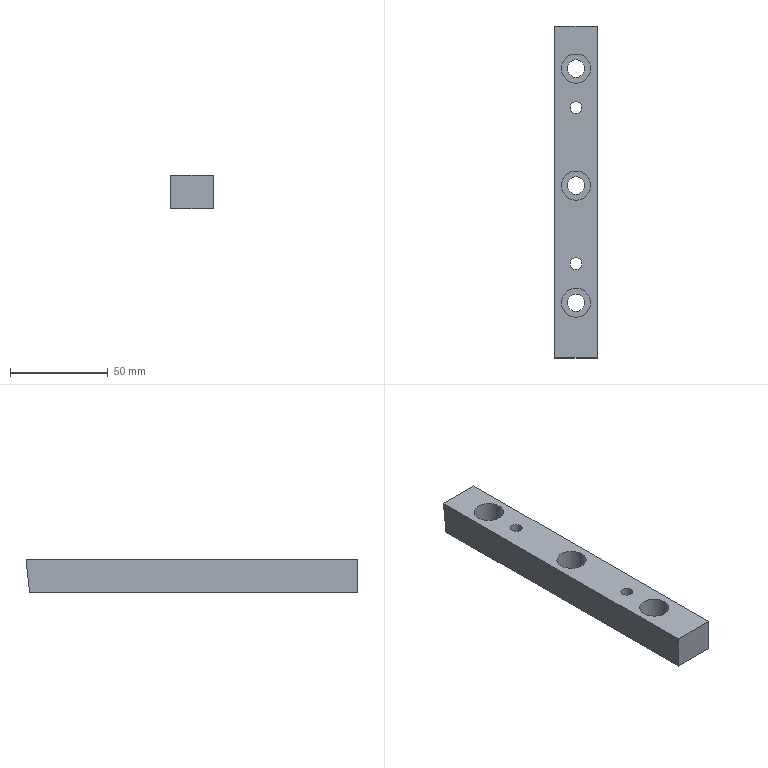Part | NX | features DATUM_CSYS 4, CBORE_HOLE 3, SKETCH 3, HOLE PACKAGE 2, SIMPLE HOLE 2, EXTRUDE 1 | 1 solid | 17 faces | box 22 x 170.1 x 17 mm | volume 55003 mm3 | plane 9 | cylinder 8 | commonest cylinder face diameters 9 x3 15 x3 6 x2
STEP:
#1=CARTESIAN_POINT('',(0.,-85.05,8.5));
#2=VERTEX_POINT('',#1);
#3=CARTESIAN_POINT('',(0.,-85.05,-8.5));
#4=VERTEX_POINT('',#3);
#5=CARTESIAN_POINT('',(0.,-85.05,8.5));
#6=DIRECTION('',(0.,0.,-1.));
#7=VECTOR('',#6,1000.);
#8=LINE('',#5,#7);
#9=EDGE_CURVE('',#2,#4,#8,.T.);
#10=ORIENTED_EDGE('',*,*,#9,.T.);
#11=CARTESIAN_POINT('',(22.,-85.05,-8.5));
#12=VERTEX_POINT('',#11);
#13=CARTESIAN_POINT('',(22.,-85.05,-8.5));
#14=DIRECTION('',(-1.,0.,0.));
#15=VECTOR('',#14,1000.);
#16=LINE('',#13,#15);
#17=EDGE_CURVE('',#12,#4,#16,.T.);
#18=ORIENTED_EDGE('',*,*,#17,.F.);
#19=CARTESIAN_POINT('',(22.,-85.05,8.5));
#20=VERTEX_POINT('',#19);
#21=CARTESIAN_POINT('',(22.,-85.05,8.5));
#22=DIRECTION('',(0.,0.,-1.));
#23=VECTOR('',#22,1000.);
#24=LINE('',#21,#23);
#25=EDGE_CURVE('',#20,#12,#24,.T.);
#26=ORIENTED_EDGE('',*,*,#25,.F.);
#27=CARTESIAN_POINT('',(22.,-85.05,8.5));
#28=DIRECTION('',(-1.,0.,0.));
#29=VECTOR('',#28,1000.);
#30=LINE('',#27,#29);
#31=EDGE_CURVE('',#20,#2,#30,.T.);
#32=ORIENTED_EDGE('',*,*,#31,.T.);
#33=EDGE_LOOP('',(#10,#18,#26,#32));
#34=FACE_BOUND('',#33,.T.);
#35=CARTESIAN_POINT('',(22.,-85.05,8.5));
#36=DIRECTION('',(0.,1.,0.));
#37=DIRECTION('',(0.,0.,1.));
#38=AXIS2_PLACEMENT_3D('',#35,#36,#37);
#39=PLANE('',#38);
#40=ADVANCED_FACE('',(#34),#39,.F.);
#41=CARTESIAN_POINT('',(14.,43.25,-8.5));
#42=VERTEX_POINT('',#41);
#43=CARTESIAN_POINT('',(11.,43.25,-8.5));
#44=DIRECTION('',(0.,0.,1.));
#45=DIRECTION('',(1.,0.,0.));
#46=AXIS2_PLACEMENT_3D('',#43,#44,#45);
#47=CIRCLE('',#46,3.);
#48=EDGE_CURVE('',#42,#42,#47,.T.);
#49=ORIENTED_EDGE('',*,*,#48,.T.);
#50=EDGE_LOOP('',(#49));
#51=FACE_BOUND('',#50,.T.);
#52=CARTESIAN_POINT('',(14.,-36.75,-8.5));
#53=VERTEX_POINT('',#52);
#54=CARTESIAN_POINT('',(11.,-36.75,-8.5));
#55=DIRECTION('',(0.,0.,1.));
#56=DIRECTION('',(1.,0.,0.));
#57=AXIS2_PLACEMENT_3D('',#54,#55,#56);
#58=CIRCLE('',#57,3.);
#59=EDGE_CURVE('',#53,#53,#58,.T.);
#60=ORIENTED_EDGE('',*,*,#59,.T.);
#61=EDGE_LOOP('',(#60));
#62=FACE_BOUND('',#61,.T.);
#63=CARTESIAN_POINT('',(15.5,63.25,-8.5));
#64=VERTEX_POINT('',#63);
#65=CARTESIAN_POINT('',(11.,63.25,-8.5));
#66=DIRECTION('',(0.,0.,1.));
#67=DIRECTION('',(1.,0.,0.));
#68=AXIS2_PLACEMENT_3D('',#65,#66,#67);
#69=CIRCLE('',#68,4.5);
#70=EDGE_CURVE('',#64,#64,#69,.T.);
#71=ORIENTED_EDGE('',*,*,#70,.T.);
#72=EDGE_LOOP('',(#71));
#73=FACE_BOUND('',#72,.T.);
#74=CARTESIAN_POINT('',(15.5,3.25,-8.5));
#75=VERTEX_POINT('',#74);
#76=CARTESIAN_POINT('',(11.,3.25,-8.5));
#77=DIRECTION('',(0.,0.,1.));
#78=DIRECTION('',(1.,0.,0.));
#79=AXIS2_PLACEMENT_3D('',#76,#77,#78);
#80=CIRCLE('',#79,4.5);
#81=EDGE_CURVE('',#75,#75,#80,.T.);
#82=ORIENTED_EDGE('',*,*,#81,.T.);
#83=EDGE_LOOP('',(#82));
#84=FACE_BOUND('',#83,.T.);
#85=CARTESIAN_POINT('',(15.5,-56.75,-8.5));
#86=VERTEX_POINT('',#85);
#87=CARTESIAN_POINT('',(11.,-56.75,-8.5));
#88=DIRECTION('',(0.,0.,1.));
#89=DIRECTION('',(1.,0.,0.));
#90=AXIS2_PLACEMENT_3D('',#87,#88,#89);
#91=CIRCLE('',#90,4.5);
#92=EDGE_CURVE('',#86,#86,#91,.T.);
#93=ORIENTED_EDGE('',*,*,#92,.T.);
#94=EDGE_LOOP('',(#93));
#95=FACE_BOUND('',#94,.T.);
#96=CARTESIAN_POINT('',(0.,83.25,-8.5));
#97=VERTEX_POINT('',#96);
#98=CARTESIAN_POINT('',(0.,-85.05,-8.5));
#99=DIRECTION('',(0.,1.,0.));
#100=VECTOR('',#99,1000.);
#101=LINE('',#98,#100);
#102=EDGE_CURVE('',#4,#97,#101,.T.);
#103=ORIENTED_EDGE('',*,*,#102,.T.);
#104=CARTESIAN_POINT('',(22.,83.25,-8.5));
#105=VERTEX_POINT('',#104);
#106=CARTESIAN_POINT('',(22.,83.25,-8.5));
#107=DIRECTION('',(-1.,0.,0.));
#108=VECTOR('',#107,1000.);
#109=LINE('',#106,#108);
#110=EDGE_CURVE('',#105,#97,#109,.T.);
#111=ORIENTED_EDGE('',*,*,#110,.F.);
#112=CARTESIAN_POINT('',(22.,-85.05,-8.5));
#113=DIRECTION('',(0.,1.,0.));
#114=VECTOR('',#113,1000.);
#115=LINE('',#112,#114);
#116=EDGE_CURVE('',#12,#105,#115,.T.);
#117=ORIENTED_EDGE('',*,*,#116,.F.);
#118=ORIENTED_EDGE('',*,*,#17,.T.);
#119=EDGE_LOOP('',(#103,#111,#117,#118));
#120=FACE_BOUND('',#119,.T.);
#121=CARTESIAN_POINT('',(22.,-85.05,-8.5));
#122=DIRECTION('',(0.,0.,1.));
#123=DIRECTION('',(1.,0.,0.));
#124=AXIS2_PLACEMENT_3D('',#121,#122,#123);
#125=PLANE('',#124);
#126=ADVANCED_FACE('',(#51,#62,#73,#84,#95,#120),#125,.F.);
#127=CARTESIAN_POINT('',(0.,85.05,8.5));
#128=VERTEX_POINT('',#127);
#129=CARTESIAN_POINT('',(0.,83.25,-8.5));
#130=DIRECTION('',(0.,0.1053,0.9944));
#131=VECTOR('',#130,1000.);
#132=LINE('',#129,#131);
#133=EDGE_CURVE('',#97,#128,#132,.T.);
#134=ORIENTED_EDGE('',*,*,#133,.T.);
#135=CARTESIAN_POINT('',(22.,85.05,8.5));
#136=VERTEX_POINT('',#135);
#137=CARTESIAN_POINT('',(22.,85.05,8.5));
#138=DIRECTION('',(-1.,0.,0.));
#139=VECTOR('',#138,1000.);
#140=LINE('',#137,#139);
#141=EDGE_CURVE('',#136,#128,#140,.T.);
#142=ORIENTED_EDGE('',*,*,#141,.F.);
#143=CARTESIAN_POINT('',(22.,83.25,-8.5));
#144=DIRECTION('',(0.,0.1053,0.9944));
#145=VECTOR('',#144,1000.);
#146=LINE('',#143,#145);
#147=EDGE_CURVE('',#105,#136,#146,.T.);
#148=ORIENTED_EDGE('',*,*,#147,.F.);
#149=ORIENTED_EDGE('',*,*,#110,.T.);
#150=EDGE_LOOP('',(#134,#142,#148,#149));
#151=FACE_BOUND('',#150,.T.);
#152=CARTESIAN_POINT('',(22.,83.25,-8.5));
#153=DIRECTION('',(0.,-0.9944,0.1053));
#154=DIRECTION('',(0.,-0.1053,-0.9944));
#155=AXIS2_PLACEMENT_3D('',#152,#153,#154);
#156=PLANE('',#155);
#157=ADVANCED_FACE('',(#151),#156,.F.);
#158=CARTESIAN_POINT('',(8.,43.25,8.5));
#159=VERTEX_POINT('',#158);
#160=CARTESIAN_POINT('',(11.,43.25,8.5));
#161=DIRECTION('',(0.,0.,-1.));
#162=DIRECTION('',(-1.,0.,0.));
#163=AXIS2_PLACEMENT_3D('',#160,#161,#162);
#164=CIRCLE('',#163,3.);
#165=EDGE_CURVE('',#159,#159,#164,.T.);
#166=ORIENTED_EDGE('',*,*,#165,.T.);
#167=EDGE_LOOP('',(#166));
#168=FACE_BOUND('',#167,.T.);
#169=CARTESIAN_POINT('',(8.,-36.75,8.5));
#170=VERTEX_POINT('',#169);
#171=CARTESIAN_POINT('',(11.,-36.75,8.5));
#172=DIRECTION('',(0.,0.,-1.));
#173=DIRECTION('',(-1.,0.,0.));
#174=AXIS2_PLACEMENT_3D('',#171,#172,#173);
#175=CIRCLE('',#174,3.);
#176=EDGE_CURVE('',#170,#170,#175,.T.);
#177=ORIENTED_EDGE('',*,*,#176,.T.);
#178=EDGE_LOOP('',(#177));
#179=FACE_BOUND('',#178,.T.);
#180=CARTESIAN_POINT('',(3.5,63.25,8.5));
#181=VERTEX_POINT('',#180);
#182=CARTESIAN_POINT('',(11.,63.25,8.5));
#183=DIRECTION('',(0.,0.,-1.));
#184=DIRECTION('',(-1.,0.,0.));
#185=AXIS2_PLACEMENT_3D('',#182,#183,#184);
#186=CIRCLE('',#185,7.5);
#187=EDGE_CURVE('',#181,#181,#186,.T.);
#188=ORIENTED_EDGE('',*,*,#187,.T.);
#189=EDGE_LOOP('',(#188));
#190=FACE_BOUND('',#189,.T.);
#191=CARTESIAN_POINT('',(3.5,3.25,8.5));
#192=VERTEX_POINT('',#191);
#193=CARTESIAN_POINT('',(11.,3.25,8.5));
#194=DIRECTION('',(0.,0.,-1.));
#195=DIRECTION('',(-1.,0.,0.));
#196=AXIS2_PLACEMENT_3D('',#193,#194,#195);
#197=CIRCLE('',#196,7.5);
#198=EDGE_CURVE('',#192,#192,#197,.T.);
#199=ORIENTED_EDGE('',*,*,#198,.T.);
#200=EDGE_LOOP('',(#199));
#201=FACE_BOUND('',#200,.T.);
#202=CARTESIAN_POINT('',(3.5,-56.75,8.5));
#203=VERTEX_POINT('',#202);
#204=CARTESIAN_POINT('',(11.,-56.75,8.5));
#205=DIRECTION('',(0.,0.,-1.));
#206=DIRECTION('',(-1.,0.,0.));
#207=AXIS2_PLACEMENT_3D('',#204,#205,#206);
#208=CIRCLE('',#207,7.5);
#209=EDGE_CURVE('',#203,#203,#208,.T.);
#210=ORIENTED_EDGE('',*,*,#209,.T.);
#211=EDGE_LOOP('',(#210));
#212=FACE_BOUND('',#211,.T.);
#213=CARTESIAN_POINT('',(0.,85.05,8.5));
#214=DIRECTION('',(0.,-1.,0.));
#215=VECTOR('',#214,1000.);
#216=LINE('',#213,#215);
#217=EDGE_CURVE('',#128,#2,#216,.T.);
#218=ORIENTED_EDGE('',*,*,#217,.T.);
#219=ORIENTED_EDGE('',*,*,#31,.F.);
#220=CARTESIAN_POINT('',(22.,85.05,8.5));
#221=DIRECTION('',(0.,-1.,0.));
#222=VECTOR('',#221,1000.);
#223=LINE('',#220,#222);
#224=EDGE_CURVE('',#136,#20,#223,.T.);
#225=ORIENTED_EDGE('',*,*,#224,.F.);
#226=ORIENTED_EDGE('',*,*,#141,.T.);
#227=EDGE_LOOP('',(#218,#219,#225,#226));
#228=FACE_BOUND('',#227,.T.);
#229=CARTESIAN_POINT('',(22.,85.05,8.5));
#230=DIRECTION('',(0.,0.,-1.));
#231=DIRECTION('',(-1.,0.,0.));
#232=AXIS2_PLACEMENT_3D('',#229,#230,#231);
#233=PLANE('',#232);
#234=ADVANCED_FACE('',(#168,#179,#190,#201,#212,#228),#233,.F.);
#235=ORIENTED_EDGE('',*,*,#25,.T.);
#236=ORIENTED_EDGE('',*,*,#116,.T.);
#237=ORIENTED_EDGE('',*,*,#147,.T.);
#238=ORIENTED_EDGE('',*,*,#224,.T.);
#239=EDGE_LOOP('',(#235,#236,#237,#238));
#240=FACE_BOUND('',#239,.T.);
#241=CARTESIAN_POINT('',(22.,0.,0.));
#242=DIRECTION('',(1.,0.,0.));
#243=DIRECTION('',(0.,0.,-1.));
#244=AXIS2_PLACEMENT_3D('',#241,#242,#243);
#245=PLANE('',#244);
#246=ADVANCED_FACE('',(#240),#245,.T.);
#247=ORIENTED_EDGE('',*,*,#9,.F.);
#248=ORIENTED_EDGE('',*,*,#217,.F.);
#249=ORIENTED_EDGE('',*,*,#133,.F.);
#250=ORIENTED_EDGE('',*,*,#102,.F.);
#251=EDGE_LOOP('',(#247,#248,#249,#250));
#252=FACE_BOUND('',#251,.T.);
#253=CARTESIAN_POINT('',(0.,0.,0.));
#254=DIRECTION('',(1.,0.,0.));
#255=DIRECTION('',(0.,0.,-1.));
#256=AXIS2_PLACEMENT_3D('',#253,#254,#255);
#257=PLANE('',#256);
#258=ADVANCED_FACE('',(#252),#257,.F.);
#259=CARTESIAN_POINT('',(6.5,-56.75,-3.5));
#260=VERTEX_POINT('',#259);
#261=CARTESIAN_POINT('',(11.,-56.75,-3.5));
#262=DIRECTION('',(0.,0.,-1.));
#263=DIRECTION('',(-1.,0.,0.));
#264=AXIS2_PLACEMENT_3D('',#261,#262,#263);
#265=CIRCLE('',#264,4.5);
#266=EDGE_CURVE('',#260,#260,#265,.F.);
#267=ORIENTED_EDGE('',*,*,#266,.T.);
#268=EDGE_LOOP('',(#267));
#269=FACE_BOUND('',#268,.T.);
#270=ORIENTED_EDGE('',*,*,#92,.F.);
#271=EDGE_LOOP('',(#270));
#272=FACE_BOUND('',#271,.T.);
#273=CARTESIAN_POINT('',(11.,-56.75,-41.5));
#274=DIRECTION('',(0.,0.,-1.));
#275=DIRECTION('',(-1.,0.,0.));
#276=AXIS2_PLACEMENT_3D('',#273,#274,#275);
#277=CYLINDRICAL_SURFACE('',#276,4.5);
#278=ADVANCED_FACE('',(#269,#272),#277,.F.);
#279=ORIENTED_EDGE('',*,*,#266,.F.);
#280=EDGE_LOOP('',(#279));
#281=FACE_BOUND('',#280,.T.);
#282=CARTESIAN_POINT('',(3.5,-56.75,-3.5));
#283=VERTEX_POINT('',#282);
#284=CARTESIAN_POINT('',(11.,-56.75,-3.5));
#285=DIRECTION('',(0.,0.,-1.));
#286=DIRECTION('',(-1.,0.,0.));
#287=AXIS2_PLACEMENT_3D('',#284,#285,#286);
#288=CIRCLE('',#287,7.5);
#289=EDGE_CURVE('',#283,#283,#288,.F.);
#290=ORIENTED_EDGE('',*,*,#289,.T.);
#291=EDGE_LOOP('',(#290));
#292=FACE_BOUND('',#291,.T.);
#293=CARTESIAN_POINT('',(11.,-56.75,-3.5));
#294=DIRECTION('',(0.,0.,-1.));
#295=DIRECTION('',(-1.,0.,0.));
#296=AXIS2_PLACEMENT_3D('',#293,#294,#295);
#297=PLANE('',#296);
#298=ADVANCED_FACE('',(#281,#292),#297,.F.);
#299=ORIENTED_EDGE('',*,*,#289,.F.);
#300=EDGE_LOOP('',(#299));
#301=FACE_BOUND('',#300,.T.);
#302=ORIENTED_EDGE('',*,*,#209,.F.);
#303=EDGE_LOOP('',(#302));
#304=FACE_BOUND('',#303,.T.);
#305=CARTESIAN_POINT('',(11.,-56.75,8.5));
#306=DIRECTION('',(0.,0.,-1.));
#307=DIRECTION('',(-1.,0.,0.));
#308=AXIS2_PLACEMENT_3D('',#305,#306,#307);
#309=CYLINDRICAL_SURFACE('',#308,7.5);
#310=ADVANCED_FACE('',(#301,#304),#309,.F.);
#311=CARTESIAN_POINT('',(6.5,3.25,-3.5));
#312=VERTEX_POINT('',#311);
#313=CARTESIAN_POINT('',(11.,3.25,-3.5));
#314=DIRECTION('',(0.,0.,-1.));
#315=DIRECTION('',(-1.,0.,0.));
#316=AXIS2_PLACEMENT_3D('',#313,#314,#315);
#317=CIRCLE('',#316,4.5);
#318=EDGE_CURVE('',#312,#312,#317,.F.);
#319=ORIENTED_EDGE('',*,*,#318,.T.);
#320=EDGE_LOOP('',(#319));
#321=FACE_BOUND('',#320,.T.);
#322=ORIENTED_EDGE('',*,*,#81,.F.);
#323=EDGE_LOOP('',(#322));
#324=FACE_BOUND('',#323,.T.);
#325=CARTESIAN_POINT('',(11.,3.25,-41.5));
#326=DIRECTION('',(0.,0.,-1.));
#327=DIRECTION('',(-1.,0.,0.));
#328=AXIS2_PLACEMENT_3D('',#325,#326,#327);
#329=CYLINDRICAL_SURFACE('',#328,4.5);
#330=ADVANCED_FACE('',(#321,#324),#329,.F.);
#331=ORIENTED_EDGE('',*,*,#318,.F.);
#332=EDGE_LOOP('',(#331));
#333=FACE_BOUND('',#332,.T.);
#334=CARTESIAN_POINT('',(3.5,3.25,-3.5));
#335=VERTEX_POINT('',#334);
#336=CARTESIAN_POINT('',(11.,3.25,-3.5));
#337=DIRECTION('',(0.,0.,-1.));
#338=DIRECTION('',(-1.,0.,0.));
#339=AXIS2_PLACEMENT_3D('',#336,#337,#338);
#340=CIRCLE('',#339,7.5);
#341=EDGE_CURVE('',#335,#335,#340,.F.);
#342=ORIENTED_EDGE('',*,*,#341,.T.);
#343=EDGE_LOOP('',(#342));
#344=FACE_BOUND('',#343,.T.);
#345=CARTESIAN_POINT('',(11.,3.25,-3.5));
#346=DIRECTION('',(0.,0.,-1.));
#347=DIRECTION('',(-1.,0.,0.));
#348=AXIS2_PLACEMENT_3D('',#345,#346,#347);
#349=PLANE('',#348);
#350=ADVANCED_FACE('',(#333,#344),#349,.F.);
#351=ORIENTED_EDGE('',*,*,#341,.F.);
#352=EDGE_LOOP('',(#351));
#353=FACE_BOUND('',#352,.T.);
#354=ORIENTED_EDGE('',*,*,#198,.F.);
#355=EDGE_LOOP('',(#354));
#356=FACE_BOUND('',#355,.T.);
#357=CARTESIAN_POINT('',(11.,3.25,8.5));
#358=DIRECTION('',(0.,0.,-1.));
#359=DIRECTION('',(-1.,0.,0.));
#360=AXIS2_PLACEMENT_3D('',#357,#358,#359);
#361=CYLINDRICAL_SURFACE('',#360,7.5);
#362=ADVANCED_FACE('',(#353,#356),#361,.F.);
#363=CARTESIAN_POINT('',(6.5,63.25,-3.5));
#364=VERTEX_POINT('',#363);
#365=CARTESIAN_POINT('',(11.,63.25,-3.5));
#366=DIRECTION('',(0.,0.,-1.));
#367=DIRECTION('',(-1.,0.,0.));
#368=AXIS2_PLACEMENT_3D('',#365,#366,#367);
#369=CIRCLE('',#368,4.5);
#370=EDGE_CURVE('',#364,#364,#369,.F.);
#371=ORIENTED_EDGE('',*,*,#370,.T.);
#372=EDGE_LOOP('',(#371));
#373=FACE_BOUND('',#372,.T.);
#374=ORIENTED_EDGE('',*,*,#70,.F.);
#375=EDGE_LOOP('',(#374));
#376=FACE_BOUND('',#375,.T.);
#377=CARTESIAN_POINT('',(11.,63.25,-41.5));
#378=DIRECTION('',(0.,0.,-1.));
#379=DIRECTION('',(-1.,0.,0.));
#380=AXIS2_PLACEMENT_3D('',#377,#378,#379);
#381=CYLINDRICAL_SURFACE('',#380,4.5);
#382=ADVANCED_FACE('',(#373,#376),#381,.F.);
#383=ORIENTED_EDGE('',*,*,#370,.F.);
#384=EDGE_LOOP('',(#383));
#385=FACE_BOUND('',#384,.T.);
#386=CARTESIAN_POINT('',(3.5,63.25,-3.5));
#387=VERTEX_POINT('',#386);
#388=CARTESIAN_POINT('',(11.,63.25,-3.5));
#389=DIRECTION('',(0.,0.,-1.));
#390=DIRECTION('',(-1.,0.,0.));
#391=AXIS2_PLACEMENT_3D('',#388,#389,#390);
#392=CIRCLE('',#391,7.5);
#393=EDGE_CURVE('',#387,#387,#392,.F.);
#394=ORIENTED_EDGE('',*,*,#393,.T.);
#395=EDGE_LOOP('',(#394));
#396=FACE_BOUND('',#395,.T.);
#397=CARTESIAN_POINT('',(11.,63.25,-3.5));
#398=DIRECTION('',(0.,0.,-1.));
#399=DIRECTION('',(-1.,0.,0.));
#400=AXIS2_PLACEMENT_3D('',#397,#398,#399);
#401=PLANE('',#400);
#402=ADVANCED_FACE('',(#385,#396),#401,.F.);
#403=ORIENTED_EDGE('',*,*,#393,.F.);
#404=EDGE_LOOP('',(#403));
#405=FACE_BOUND('',#404,.T.);
#406=ORIENTED_EDGE('',*,*,#187,.F.);
#407=EDGE_LOOP('',(#406));
#408=FACE_BOUND('',#407,.T.);
#409=CARTESIAN_POINT('',(11.,63.25,8.5));
#410=DIRECTION('',(0.,0.,-1.));
#411=DIRECTION('',(-1.,0.,0.));
#412=AXIS2_PLACEMENT_3D('',#409,#410,#411);
#413=CYLINDRICAL_SURFACE('',#412,7.5);
#414=ADVANCED_FACE('',(#405,#408),#413,.F.);
#415=ORIENTED_EDGE('',*,*,#176,.F.);
#416=EDGE_LOOP('',(#415));
#417=FACE_BOUND('',#416,.T.);
#418=ORIENTED_EDGE('',*,*,#59,.F.);
#419=EDGE_LOOP('',(#418));
#420=FACE_BOUND('',#419,.T.);
#421=CARTESIAN_POINT('',(11.,-36.75,8.5));
#422=DIRECTION('',(0.,0.,-1.));
#423=DIRECTION('',(-1.,0.,0.));
#424=AXIS2_PLACEMENT_3D('',#421,#422,#423);
#425=CYLINDRICAL_SURFACE('',#424,3.);
#426=ADVANCED_FACE('',(#417,#420),#425,.F.);
#427=ORIENTED_EDGE('',*,*,#165,.F.);
#428=EDGE_LOOP('',(#427));
#429=FACE_BOUND('',#428,.T.);
#430=ORIENTED_EDGE('',*,*,#48,.F.);
#431=EDGE_LOOP('',(#430));
#432=FACE_BOUND('',#431,.T.);
#433=CARTESIAN_POINT('',(11.,43.25,8.5));
#434=DIRECTION('',(0.,0.,-1.));
#435=DIRECTION('',(-1.,0.,0.));
#436=AXIS2_PLACEMENT_3D('',#433,#434,#435);
#437=CYLINDRICAL_SURFACE('',#436,3.);
#438=ADVANCED_FACE('',(#429,#432),#437,.F.);
#439=CLOSED_SHELL('',(#40,#126,#157,#234,#246,#258,#278,#298,#310,#330,#350,#362,#382,#402,#414,#426,#438));
#440=MANIFOLD_SOLID_BREP('',#439);
#441=(LENGTH_UNIT()NAMED_UNIT(*)SI_UNIT(.MILLI.,.METRE.));
#442=UNCERTAINTY_MEASURE_WITH_UNIT(LENGTH_MEASURE(0.00001),#441,'','');
#443=(NAMED_UNIT(*)PLANE_ANGLE_UNIT()SI_UNIT($,.RADIAN.));
#444=(NAMED_UNIT(*)SI_UNIT($,.STERADIAN.)SOLID_ANGLE_UNIT());
#445=(GEOMETRIC_REPRESENTATION_CONTEXT(3)GLOBAL_UNCERTAINTY_ASSIGNED_CONTEXT((#442))GLOBAL_UNIT_ASSIGNED_CONTEXT((#441,#443,#444))REPRESENTATION_CONTEXT('',''));
#446=ADVANCED_BREP_SHAPE_REPRESENTATION('',(#440),#445);